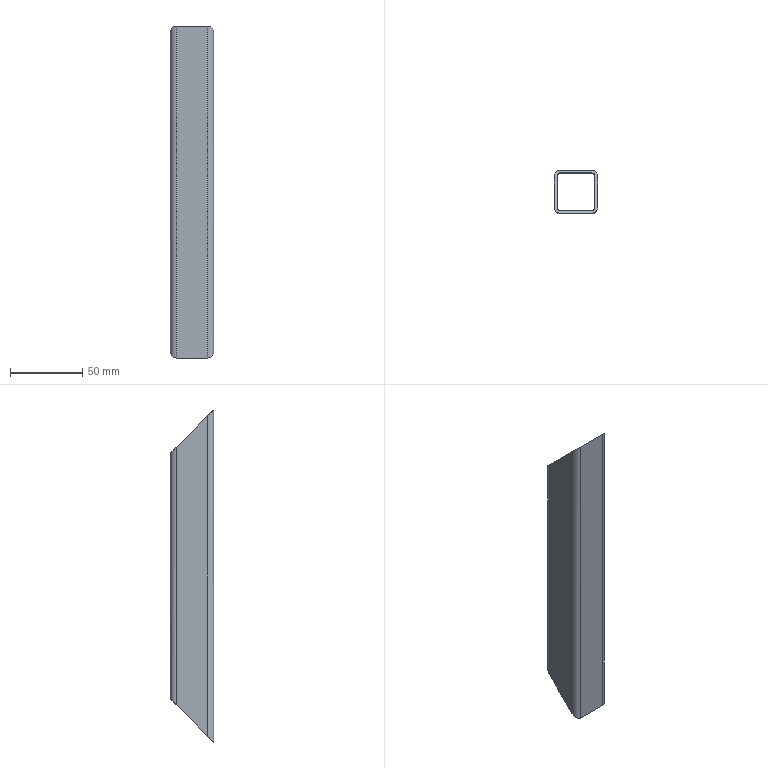Part | NX | features DATUM_CSYS 3, EXTRUDE 2, SKETCH 2, CPROJ 1 | 1 solid | 18 faces | box 30 x 30 x 230 mm | volume 42740 mm3 | plane 10 | cylinder 8 | commonest cylinder face diameters 4 x4 8 x4
STEP:
#1=CARTESIAN_POINT('',(13.,11.,26.));
#2=VERTEX_POINT('',#1);
#3=CARTESIAN_POINT('',(13.,11.,204.));
#4=VERTEX_POINT('',#3);
#5=CARTESIAN_POINT('',(13.,11.,0.));
#6=DIRECTION('',(0.,0.,-1.));
#7=VECTOR('',#6,1000.);
#8=LINE('',#5,#7);
#9=EDGE_CURVE('',#2,#4,#8,.F.);
#10=ORIENTED_EDGE('',*,*,#9,.T.);
#11=CARTESIAN_POINT('',(11.,13.,202.));
#12=VERTEX_POINT('',#11);
#13=CARTESIAN_POINT('',(11.,11.,204.));
#14=DIRECTION('',(0.,-0.7071,-0.7071));
#15=DIRECTION('',(0.,-0.7071,0.7071));
#16=AXIS2_PLACEMENT_3D('',#13,#14,#15);
#17=ELLIPSE('',#16,2.828,2.);
#18=EDGE_CURVE('',#4,#12,#17,.F.);
#19=ORIENTED_EDGE('',*,*,#18,.T.);
#20=CARTESIAN_POINT('',(11.,13.,28.));
#21=VERTEX_POINT('',#20);
#22=CARTESIAN_POINT('',(11.,13.,0.));
#23=DIRECTION('',(0.,0.,1.));
#24=VECTOR('',#23,1000.);
#25=LINE('',#22,#24);
#26=EDGE_CURVE('',#21,#12,#25,.T.);
#27=ORIENTED_EDGE('',*,*,#26,.F.);
#28=CARTESIAN_POINT('',(11.,11.,26.));
#29=DIRECTION('',(0.,-0.7071,0.7071));
#30=DIRECTION('',(0.,0.7071,0.7071));
#31=AXIS2_PLACEMENT_3D('',#28,#29,#30);
#32=ELLIPSE('',#31,2.828,2.);
#33=EDGE_CURVE('',#21,#2,#32,.F.);
#34=ORIENTED_EDGE('',*,*,#33,.T.);
#35=EDGE_LOOP('',(#10,#19,#27,#34));
#36=FACE_BOUND('',#35,.T.);
#37=CARTESIAN_POINT('',(11.,11.,0.));
#38=DIRECTION('',(0.,0.,1.));
#39=DIRECTION('',(1.,0.,0.));
#40=AXIS2_PLACEMENT_3D('',#37,#38,#39);
#41=CYLINDRICAL_SURFACE('',#40,2.);
#42=ADVANCED_FACE('',(#36),#41,.F.);
#43=CARTESIAN_POINT('',(13.,-11.,4.));
#44=VERTEX_POINT('',#43);
#45=CARTESIAN_POINT('',(13.,-11.,226.));
#46=VERTEX_POINT('',#45);
#47=CARTESIAN_POINT('',(13.,-11.,0.));
#48=DIRECTION('',(0.,0.,1.));
#49=VECTOR('',#48,1000.);
#50=LINE('',#47,#49);
#51=EDGE_CURVE('',#44,#46,#50,.T.);
#52=ORIENTED_EDGE('',*,*,#51,.T.);
#53=CARTESIAN_POINT('',(13.,102.,113.));
#54=DIRECTION('',(0.,0.7071,-0.7071));
#55=VECTOR('',#54,1000.);
#56=LINE('',#53,#55);
#57=EDGE_CURVE('',#46,#4,#56,.T.);
#58=ORIENTED_EDGE('',*,*,#57,.T.);
#59=ORIENTED_EDGE('',*,*,#9,.F.);
#60=CARTESIAN_POINT('',(13.,-13.,2.));
#61=DIRECTION('',(0.,-0.7071,-0.7071));
#62=VECTOR('',#61,1000.);
#63=LINE('',#60,#62);
#64=EDGE_CURVE('',#2,#44,#63,.T.);
#65=ORIENTED_EDGE('',*,*,#64,.T.);
#66=EDGE_LOOP('',(#52,#58,#59,#65));
#67=FACE_BOUND('',#66,.T.);
#68=CARTESIAN_POINT('',(13.,-11.,0.));
#69=DIRECTION('',(1.,0.,0.));
#70=DIRECTION('',(0.,0.,-1.));
#71=AXIS2_PLACEMENT_3D('',#68,#69,#70);
#72=PLANE('',#71);
#73=ADVANCED_FACE('',(#67),#72,.F.);
#74=CARTESIAN_POINT('',(11.,-13.,2.));
#75=VERTEX_POINT('',#74);
#76=CARTESIAN_POINT('',(11.,-13.,228.));
#77=VERTEX_POINT('',#76);
#78=CARTESIAN_POINT('',(11.,-13.,0.));
#79=DIRECTION('',(0.,0.,1.));
#80=VECTOR('',#79,1000.);
#81=LINE('',#78,#80);
#82=EDGE_CURVE('',#75,#77,#81,.T.);
#83=ORIENTED_EDGE('',*,*,#82,.T.);
#84=CARTESIAN_POINT('',(11.,-11.,226.));
#85=DIRECTION('',(0.,-0.7071,-0.7071));
#86=DIRECTION('',(0.,-0.7071,0.7071));
#87=AXIS2_PLACEMENT_3D('',#84,#85,#86);
#88=ELLIPSE('',#87,2.828,2.);
#89=EDGE_CURVE('',#77,#46,#88,.F.);
#90=ORIENTED_EDGE('',*,*,#89,.T.);
#91=ORIENTED_EDGE('',*,*,#51,.F.);
#92=CARTESIAN_POINT('',(11.,-11.,4.));
#93=DIRECTION('',(0.,-0.7071,0.7071));
#94=DIRECTION('',(0.,0.7071,0.7071));
#95=AXIS2_PLACEMENT_3D('',#92,#93,#94);
#96=ELLIPSE('',#95,2.828,2.);
#97=EDGE_CURVE('',#44,#75,#96,.F.);
#98=ORIENTED_EDGE('',*,*,#97,.T.);
#99=EDGE_LOOP('',(#83,#90,#91,#98));
#100=FACE_BOUND('',#99,.T.);
#101=CARTESIAN_POINT('',(11.,-11.,0.));
#102=DIRECTION('',(0.,0.,1.));
#103=DIRECTION('',(1.,0.,0.));
#104=AXIS2_PLACEMENT_3D('',#101,#102,#103);
#105=CYLINDRICAL_SURFACE('',#104,2.);
#106=ADVANCED_FACE('',(#100),#105,.F.);
#107=CARTESIAN_POINT('',(-11.,-13.,2.));
#108=VERTEX_POINT('',#107);
#109=CARTESIAN_POINT('',(-11.,-13.,228.));
#110=VERTEX_POINT('',#109);
#111=CARTESIAN_POINT('',(-11.,-13.,0.));
#112=DIRECTION('',(0.,0.,1.));
#113=VECTOR('',#112,1000.);
#114=LINE('',#111,#113);
#115=EDGE_CURVE('',#108,#110,#114,.T.);
#116=ORIENTED_EDGE('',*,*,#115,.T.);
#117=CARTESIAN_POINT('',(-11.,-13.,228.));
#118=DIRECTION('',(1.,0.,0.));
#119=VECTOR('',#118,1000.);
#120=LINE('',#117,#119);
#121=EDGE_CURVE('',#110,#77,#120,.T.);
#122=ORIENTED_EDGE('',*,*,#121,.T.);
#123=ORIENTED_EDGE('',*,*,#82,.F.);
#124=CARTESIAN_POINT('',(-11.,-13.,2.));
#125=DIRECTION('',(-1.,0.,0.));
#126=VECTOR('',#125,1000.);
#127=LINE('',#124,#126);
#128=EDGE_CURVE('',#75,#108,#127,.T.);
#129=ORIENTED_EDGE('',*,*,#128,.T.);
#130=EDGE_LOOP('',(#116,#122,#123,#129));
#131=FACE_BOUND('',#130,.T.);
#132=CARTESIAN_POINT('',(-11.,-13.,0.));
#133=DIRECTION('',(0.,-1.,0.));
#134=DIRECTION('',(1.,0.,0.));
#135=AXIS2_PLACEMENT_3D('',#132,#133,#134);
#136=PLANE('',#135);
#137=ADVANCED_FACE('',(#131),#136,.F.);
#138=CARTESIAN_POINT('',(-13.,-11.,4.));
#139=VERTEX_POINT('',#138);
#140=CARTESIAN_POINT('',(-13.,-11.,226.));
#141=VERTEX_POINT('',#140);
#142=CARTESIAN_POINT('',(-13.,-11.,0.));
#143=DIRECTION('',(0.,0.,1.));
#144=VECTOR('',#143,1000.);
#145=LINE('',#142,#144);
#146=EDGE_CURVE('',#139,#141,#145,.T.);
#147=ORIENTED_EDGE('',*,*,#146,.T.);
#148=CARTESIAN_POINT('',(-11.,-11.,226.));
#149=DIRECTION('',(0.,-0.7071,-0.7071));
#150=DIRECTION('',(0.,-0.7071,0.7071));
#151=AXIS2_PLACEMENT_3D('',#148,#149,#150);
#152=ELLIPSE('',#151,2.828,2.);
#153=EDGE_CURVE('',#141,#110,#152,.F.);
#154=ORIENTED_EDGE('',*,*,#153,.T.);
#155=ORIENTED_EDGE('',*,*,#115,.F.);
#156=CARTESIAN_POINT('',(-11.,-11.,4.));
#157=DIRECTION('',(0.,-0.7071,0.7071));
#158=DIRECTION('',(0.,0.7071,0.7071));
#159=AXIS2_PLACEMENT_3D('',#156,#157,#158);
#160=ELLIPSE('',#159,2.828,2.);
#161=EDGE_CURVE('',#108,#139,#160,.F.);
#162=ORIENTED_EDGE('',*,*,#161,.T.);
#163=EDGE_LOOP('',(#147,#154,#155,#162));
#164=FACE_BOUND('',#163,.T.);
#165=CARTESIAN_POINT('',(-11.,-11.,0.));
#166=DIRECTION('',(0.,0.,1.));
#167=DIRECTION('',(1.,0.,0.));
#168=AXIS2_PLACEMENT_3D('',#165,#166,#167);
#169=CYLINDRICAL_SURFACE('',#168,2.);
#170=ADVANCED_FACE('',(#164),#169,.F.);
#171=CARTESIAN_POINT('',(-13.,11.,26.));
#172=VERTEX_POINT('',#171);
#173=CARTESIAN_POINT('',(-13.,11.,204.));
#174=VERTEX_POINT('',#173);
#175=CARTESIAN_POINT('',(-13.,11.,0.));
#176=DIRECTION('',(0.,0.,1.));
#177=VECTOR('',#176,1000.);
#178=LINE('',#175,#177);
#179=EDGE_CURVE('',#172,#174,#178,.T.);
#180=ORIENTED_EDGE('',*,*,#179,.T.);
#181=CARTESIAN_POINT('',(-13.,113.,102.));
#182=DIRECTION('',(0.,-0.7071,0.7071));
#183=VECTOR('',#182,1000.);
#184=LINE('',#181,#183);
#185=EDGE_CURVE('',#174,#141,#184,.T.);
#186=ORIENTED_EDGE('',*,*,#185,.T.);
#187=ORIENTED_EDGE('',*,*,#146,.F.);
#188=CARTESIAN_POINT('',(-13.,-2.,13.));
#189=DIRECTION('',(0.,0.7071,0.7071));
#190=VECTOR('',#189,1000.);
#191=LINE('',#188,#190);
#192=EDGE_CURVE('',#139,#172,#191,.T.);
#193=ORIENTED_EDGE('',*,*,#192,.T.);
#194=EDGE_LOOP('',(#180,#186,#187,#193));
#195=FACE_BOUND('',#194,.T.);
#196=CARTESIAN_POINT('',(-13.,11.,0.));
#197=DIRECTION('',(-1.,0.,0.));
#198=DIRECTION('',(0.,-1.,0.));
#199=AXIS2_PLACEMENT_3D('',#196,#197,#198);
#200=PLANE('',#199);
#201=ADVANCED_FACE('',(#195),#200,.F.);
#202=CARTESIAN_POINT('',(-11.,13.,28.));
#203=VERTEX_POINT('',#202);
#204=CARTESIAN_POINT('',(-11.,13.,202.));
#205=VERTEX_POINT('',#204);
#206=CARTESIAN_POINT('',(-11.,13.,0.));
#207=DIRECTION('',(0.,0.,1.));
#208=VECTOR('',#207,1000.);
#209=LINE('',#206,#208);
#210=EDGE_CURVE('',#203,#205,#209,.T.);
#211=ORIENTED_EDGE('',*,*,#210,.T.);
#212=CARTESIAN_POINT('',(-11.,11.,204.));
#213=DIRECTION('',(0.,-0.7071,-0.7071));
#214=DIRECTION('',(0.,-0.7071,0.7071));
#215=AXIS2_PLACEMENT_3D('',#212,#213,#214);
#216=ELLIPSE('',#215,2.828,2.);
#217=EDGE_CURVE('',#205,#174,#216,.F.);
#218=ORIENTED_EDGE('',*,*,#217,.T.);
#219=ORIENTED_EDGE('',*,*,#179,.F.);
#220=CARTESIAN_POINT('',(-11.,11.,26.));
#221=DIRECTION('',(0.,-0.7071,0.7071));
#222=DIRECTION('',(0.,0.7071,0.7071));
#223=AXIS2_PLACEMENT_3D('',#220,#221,#222);
#224=ELLIPSE('',#223,2.828,2.);
#225=EDGE_CURVE('',#172,#203,#224,.F.);
#226=ORIENTED_EDGE('',*,*,#225,.T.);
#227=EDGE_LOOP('',(#211,#218,#219,#226));
#228=FACE_BOUND('',#227,.T.);
#229=CARTESIAN_POINT('',(-11.,11.,0.));
#230=DIRECTION('',(0.,0.,1.));
#231=DIRECTION('',(1.,0.,0.));
#232=AXIS2_PLACEMENT_3D('',#229,#230,#231);
#233=CYLINDRICAL_SURFACE('',#232,2.);
#234=ADVANCED_FACE('',(#228),#233,.F.);
#235=ORIENTED_EDGE('',*,*,#26,.T.);
#236=CARTESIAN_POINT('',(11.,13.,202.));
#237=DIRECTION('',(-1.,0.,0.));
#238=VECTOR('',#237,1000.);
#239=LINE('',#236,#238);
#240=EDGE_CURVE('',#12,#205,#239,.T.);
#241=ORIENTED_EDGE('',*,*,#240,.T.);
#242=ORIENTED_EDGE('',*,*,#210,.F.);
#243=CARTESIAN_POINT('',(11.,13.,28.));
#244=DIRECTION('',(1.,0.,0.));
#245=VECTOR('',#244,1000.);
#246=LINE('',#243,#245);
#247=EDGE_CURVE('',#203,#21,#246,.T.);
#248=ORIENTED_EDGE('',*,*,#247,.T.);
#249=EDGE_LOOP('',(#235,#241,#242,#248));
#250=FACE_BOUND('',#249,.T.);
#251=CARTESIAN_POINT('',(11.,13.,0.));
#252=DIRECTION('',(0.,1.,0.));
#253=DIRECTION('',(-1.,0.,0.));
#254=AXIS2_PLACEMENT_3D('',#251,#252,#253);
#255=PLANE('',#254);
#256=ADVANCED_FACE('',(#250),#255,.F.);
#257=CARTESIAN_POINT('',(-15.,11.,26.));
#258=VERTEX_POINT('',#257);
#259=CARTESIAN_POINT('',(-11.,15.,30.));
#260=VERTEX_POINT('',#259);
#261=CARTESIAN_POINT('',(-11.,11.,26.));
#262=DIRECTION('',(0.,-0.7071,0.7071));
#263=DIRECTION('',(0.,0.7071,0.7071));
#264=AXIS2_PLACEMENT_3D('',#261,#262,#263);
#265=ELLIPSE('',#264,5.657,4.);
#266=EDGE_CURVE('',#258,#260,#265,.F.);
#267=ORIENTED_EDGE('',*,*,#266,.T.);
#268=CARTESIAN_POINT('',(11.,15.,30.));
#269=VERTEX_POINT('',#268);
#270=CARTESIAN_POINT('',(-29.5,15.,30.));
#271=DIRECTION('',(1.,0.,0.));
#272=VECTOR('',#271,1000.);
#273=LINE('',#270,#272);
#274=EDGE_CURVE('',#260,#269,#273,.T.);
#275=ORIENTED_EDGE('',*,*,#274,.T.);
#276=CARTESIAN_POINT('',(15.,11.,26.));
#277=VERTEX_POINT('',#276);
#278=CARTESIAN_POINT('',(11.,11.,26.));
#279=DIRECTION('',(0.,-0.7071,0.7071));
#280=DIRECTION('',(0.,0.7071,0.7071));
#281=AXIS2_PLACEMENT_3D('',#278,#279,#280);
#282=ELLIPSE('',#281,5.657,4.);
#283=EDGE_CURVE('',#269,#277,#282,.F.);
#284=ORIENTED_EDGE('',*,*,#283,.T.);
#285=CARTESIAN_POINT('',(15.,-11.,4.));
#286=VERTEX_POINT('',#285);
#287=CARTESIAN_POINT('',(15.,15.,30.));
#288=DIRECTION('',(0.,-0.7071,-0.7071));
#289=VECTOR('',#288,1000.);
#290=LINE('',#287,#289);
#291=EDGE_CURVE('',#277,#286,#290,.T.);
#292=ORIENTED_EDGE('',*,*,#291,.T.);
#293=CARTESIAN_POINT('',(11.,-15.,0.));
#294=VERTEX_POINT('',#293);
#295=CARTESIAN_POINT('',(11.,-11.,4.));
#296=DIRECTION('',(0.,-0.7071,0.7071));
#297=DIRECTION('',(0.,0.7071,0.7071));
#298=AXIS2_PLACEMENT_3D('',#295,#296,#297);
#299=ELLIPSE('',#298,5.657,4.);
#300=EDGE_CURVE('',#286,#294,#299,.F.);
#301=ORIENTED_EDGE('',*,*,#300,.T.);
#302=CARTESIAN_POINT('',(-11.,-15.,0.));
#303=VERTEX_POINT('',#302);
#304=CARTESIAN_POINT('',(-11.,-15.,0.));
#305=DIRECTION('',(1.,0.,0.));
#306=VECTOR('',#305,1000.);
#307=LINE('',#304,#306);
#308=EDGE_CURVE('',#303,#294,#307,.T.);
#309=ORIENTED_EDGE('',*,*,#308,.F.);
#310=CARTESIAN_POINT('',(-15.,-11.,4.));
#311=VERTEX_POINT('',#310);
#312=CARTESIAN_POINT('',(-11.,-11.,4.));
#313=DIRECTION('',(0.,-0.7071,0.7071));
#314=DIRECTION('',(0.,0.7071,0.7071));
#315=AXIS2_PLACEMENT_3D('',#312,#313,#314);
#316=ELLIPSE('',#315,5.657,4.);
#317=EDGE_CURVE('',#303,#311,#316,.F.);
#318=ORIENTED_EDGE('',*,*,#317,.T.);
#319=CARTESIAN_POINT('',(-15.,-2.,13.));
#320=DIRECTION('',(0.,0.7071,0.7071));
#321=VECTOR('',#320,1000.);
#322=LINE('',#319,#321);
#323=EDGE_CURVE('',#311,#258,#322,.T.);
#324=ORIENTED_EDGE('',*,*,#323,.T.);
#325=EDGE_LOOP('',(#267,#275,#284,#292,#301,#309,#318,#324));
#326=FACE_BOUND('',#325,.T.);
#327=ORIENTED_EDGE('',*,*,#225,.F.);
#328=ORIENTED_EDGE('',*,*,#192,.F.);
#329=ORIENTED_EDGE('',*,*,#161,.F.);
#330=ORIENTED_EDGE('',*,*,#128,.F.);
#331=ORIENTED_EDGE('',*,*,#97,.F.);
#332=ORIENTED_EDGE('',*,*,#64,.F.);
#333=ORIENTED_EDGE('',*,*,#33,.F.);
#334=ORIENTED_EDGE('',*,*,#247,.F.);
#335=EDGE_LOOP('',(#327,#328,#329,#330,#331,#332,#333,#334));
#336=FACE_BOUND('',#335,.T.);
#337=CARTESIAN_POINT('',(-29.5,15.,30.));
#338=DIRECTION('',(0.,-0.7071,0.7071));
#339=DIRECTION('',(0.,-0.7071,-0.7071));
#340=AXIS2_PLACEMENT_3D('',#337,#338,#339);
#341=PLANE('',#340);
#342=ADVANCED_FACE('',(#326,#336),#341,.F.);
#343=CARTESIAN_POINT('',(-11.,15.,200.));
#344=VERTEX_POINT('',#343);
#345=CARTESIAN_POINT('',(-15.,11.,204.));
#346=VERTEX_POINT('',#345);
#347=CARTESIAN_POINT('',(-11.,11.,204.));
#348=DIRECTION('',(0.,-0.7071,-0.7071));
#349=DIRECTION('',(0.,-0.7071,0.7071));
#350=AXIS2_PLACEMENT_3D('',#347,#348,#349);
#351=ELLIPSE('',#350,5.657,4.);
#352=EDGE_CURVE('',#344,#346,#351,.F.);
#353=ORIENTED_EDGE('',*,*,#352,.T.);
#354=CARTESIAN_POINT('',(-15.,-11.,226.));
#355=VERTEX_POINT('',#354);
#356=CARTESIAN_POINT('',(-15.,113.,102.));
#357=DIRECTION('',(0.,-0.7071,0.7071));
#358=VECTOR('',#357,1000.);
#359=LINE('',#356,#358);
#360=EDGE_CURVE('',#346,#355,#359,.T.);
#361=ORIENTED_EDGE('',*,*,#360,.T.);
#362=CARTESIAN_POINT('',(-11.,-15.,230.));
#363=VERTEX_POINT('',#362);
#364=CARTESIAN_POINT('',(-11.,-11.,226.));
#365=DIRECTION('',(0.,-0.7071,-0.7071));
#366=DIRECTION('',(0.,-0.7071,0.7071));
#367=AXIS2_PLACEMENT_3D('',#364,#365,#366);
#368=ELLIPSE('',#367,5.657,4.);
#369=EDGE_CURVE('',#355,#363,#368,.F.);
#370=ORIENTED_EDGE('',*,*,#369,.T.);
#371=CARTESIAN_POINT('',(11.,-15.,230.));
#372=VERTEX_POINT('',#371);
#373=CARTESIAN_POINT('',(-11.,-15.,230.));
#374=DIRECTION('',(1.,0.,0.));
#375=VECTOR('',#374,1000.);
#376=LINE('',#373,#375);
#377=EDGE_CURVE('',#363,#372,#376,.T.);
#378=ORIENTED_EDGE('',*,*,#377,.T.);
#379=CARTESIAN_POINT('',(15.,-11.,226.));
#380=VERTEX_POINT('',#379);
#381=CARTESIAN_POINT('',(11.,-11.,226.));
#382=DIRECTION('',(0.,-0.7071,-0.7071));
#383=DIRECTION('',(0.,-0.7071,0.7071));
#384=AXIS2_PLACEMENT_3D('',#381,#382,#383);
#385=ELLIPSE('',#384,5.657,4.);
#386=EDGE_CURVE('',#372,#380,#385,.F.);
#387=ORIENTED_EDGE('',*,*,#386,.T.);
#388=CARTESIAN_POINT('',(15.,11.,204.));
#389=VERTEX_POINT('',#388);
#390=CARTESIAN_POINT('',(15.,-15.,230.));
#391=DIRECTION('',(0.,0.7071,-0.7071));
#392=VECTOR('',#391,1000.);
#393=LINE('',#390,#392);
#394=EDGE_CURVE('',#380,#389,#393,.T.);
#395=ORIENTED_EDGE('',*,*,#394,.T.);
#396=CARTESIAN_POINT('',(11.,15.,200.));
#397=VERTEX_POINT('',#396);
#398=CARTESIAN_POINT('',(11.,11.,204.));
#399=DIRECTION('',(0.,-0.7071,-0.7071));
#400=DIRECTION('',(0.,-0.7071,0.7071));
#401=AXIS2_PLACEMENT_3D('',#398,#399,#400);
#402=ELLIPSE('',#401,5.657,4.);
#403=EDGE_CURVE('',#389,#397,#402,.F.);
#404=ORIENTED_EDGE('',*,*,#403,.T.);
#405=CARTESIAN_POINT('',(-29.5,15.,200.));
#406=DIRECTION('',(1.,0.,0.));
#407=VECTOR('',#406,1000.);
#408=LINE('',#405,#407);
#409=EDGE_CURVE('',#344,#397,#408,.T.);
#410=ORIENTED_EDGE('',*,*,#409,.F.);
#411=EDGE_LOOP('',(#353,#361,#370,#378,#387,#395,#404,#410));
#412=FACE_BOUND('',#411,.T.);
#413=ORIENTED_EDGE('',*,*,#18,.F.);
#414=ORIENTED_EDGE('',*,*,#57,.F.);
#415=ORIENTED_EDGE('',*,*,#89,.F.);
#416=ORIENTED_EDGE('',*,*,#121,.F.);
#417=ORIENTED_EDGE('',*,*,#153,.F.);
#418=ORIENTED_EDGE('',*,*,#185,.F.);
#419=ORIENTED_EDGE('',*,*,#217,.F.);
#420=ORIENTED_EDGE('',*,*,#240,.F.);
#421=EDGE_LOOP('',(#413,#414,#415,#416,#417,#418,#419,#420));
#422=FACE_BOUND('',#421,.T.);
#423=CARTESIAN_POINT('',(-29.5,-15.,230.));
#424=DIRECTION('',(0.,-0.7071,-0.7071));
#425=DIRECTION('',(0.,0.7071,-0.7071));
#426=AXIS2_PLACEMENT_3D('',#423,#424,#425);
#427=PLANE('',#426);
#428=ADVANCED_FACE('',(#412,#422),#427,.F.);
#429=CARTESIAN_POINT('',(-11.,15.,0.));
#430=DIRECTION('',(0.,0.,1.));
#431=VECTOR('',#430,1000.);
#432=LINE('',#429,#431);
#433=EDGE_CURVE('',#260,#344,#432,.T.);
#434=ORIENTED_EDGE('',*,*,#433,.T.);
#435=ORIENTED_EDGE('',*,*,#409,.T.);
#436=CARTESIAN_POINT('',(11.,15.,0.));
#437=DIRECTION('',(0.,0.,1.));
#438=VECTOR('',#437,1000.);
#439=LINE('',#436,#438);
#440=EDGE_CURVE('',#269,#397,#439,.T.);
#441=ORIENTED_EDGE('',*,*,#440,.F.);
#442=ORIENTED_EDGE('',*,*,#274,.F.);
#443=EDGE_LOOP('',(#434,#435,#441,#442));
#444=FACE_BOUND('',#443,.T.);
#445=CARTESIAN_POINT('',(11.,15.,0.));
#446=DIRECTION('',(0.,1.,0.));
#447=DIRECTION('',(-1.,0.,0.));
#448=AXIS2_PLACEMENT_3D('',#445,#446,#447);
#449=PLANE('',#448);
#450=ADVANCED_FACE('',(#444),#449,.T.);
#451=ORIENTED_EDGE('',*,*,#352,.F.);
#452=ORIENTED_EDGE('',*,*,#433,.F.);
#453=ORIENTED_EDGE('',*,*,#266,.F.);
#454=CARTESIAN_POINT('',(-15.,11.,0.));
#455=DIRECTION('',(0.,0.,1.));
#456=VECTOR('',#455,1000.);
#457=LINE('',#454,#456);
#458=EDGE_CURVE('',#258,#346,#457,.T.);
#459=ORIENTED_EDGE('',*,*,#458,.T.);
#460=EDGE_LOOP('',(#451,#452,#453,#459));
#461=FACE_BOUND('',#460,.T.);
#462=CARTESIAN_POINT('',(-11.,11.,0.));
#463=DIRECTION('',(0.,0.,1.));
#464=DIRECTION('',(1.,0.,0.));
#465=AXIS2_PLACEMENT_3D('',#462,#463,#464);
#466=CYLINDRICAL_SURFACE('',#465,4.);
#467=ADVANCED_FACE('',(#461),#466,.T.);
#468=ORIENTED_EDGE('',*,*,#360,.F.);
#469=ORIENTED_EDGE('',*,*,#458,.F.);
#470=ORIENTED_EDGE('',*,*,#323,.F.);
#471=CARTESIAN_POINT('',(-15.,-11.,0.));
#472=DIRECTION('',(0.,0.,1.));
#473=VECTOR('',#472,1000.);
#474=LINE('',#471,#473);
#475=EDGE_CURVE('',#311,#355,#474,.T.);
#476=ORIENTED_EDGE('',*,*,#475,.T.);
#477=EDGE_LOOP('',(#468,#469,#470,#476));
#478=FACE_BOUND('',#477,.T.);
#479=CARTESIAN_POINT('',(-15.,11.,0.));
#480=DIRECTION('',(-1.,0.,0.));
#481=DIRECTION('',(0.,-1.,0.));
#482=AXIS2_PLACEMENT_3D('',#479,#480,#481);
#483=PLANE('',#482);
#484=ADVANCED_FACE('',(#478),#483,.T.);
#485=ORIENTED_EDGE('',*,*,#369,.F.);
#486=ORIENTED_EDGE('',*,*,#475,.F.);
#487=ORIENTED_EDGE('',*,*,#317,.F.);
#488=CARTESIAN_POINT('',(-11.,-15.,0.));
#489=DIRECTION('',(0.,0.,1.));
#490=VECTOR('',#489,1000.);
#491=LINE('',#488,#490);
#492=EDGE_CURVE('',#303,#363,#491,.T.);
#493=ORIENTED_EDGE('',*,*,#492,.T.);
#494=EDGE_LOOP('',(#485,#486,#487,#493));
#495=FACE_BOUND('',#494,.T.);
#496=CARTESIAN_POINT('',(-11.,-11.,0.));
#497=DIRECTION('',(0.,0.,1.));
#498=DIRECTION('',(1.,0.,0.));
#499=AXIS2_PLACEMENT_3D('',#496,#497,#498);
#500=CYLINDRICAL_SURFACE('',#499,4.);
#501=ADVANCED_FACE('',(#495),#500,.T.);
#502=ORIENTED_EDGE('',*,*,#377,.F.);
#503=ORIENTED_EDGE('',*,*,#492,.F.);
#504=ORIENTED_EDGE('',*,*,#308,.T.);
#505=CARTESIAN_POINT('',(11.,-15.,0.));
#506=DIRECTION('',(0.,0.,1.));
#507=VECTOR('',#506,1000.);
#508=LINE('',#505,#507);
#509=EDGE_CURVE('',#294,#372,#508,.T.);
#510=ORIENTED_EDGE('',*,*,#509,.T.);
#511=EDGE_LOOP('',(#502,#503,#504,#510));
#512=FACE_BOUND('',#511,.T.);
#513=CARTESIAN_POINT('',(-11.,-15.,0.));
#514=DIRECTION('',(0.,-1.,0.));
#515=DIRECTION('',(1.,0.,0.));
#516=AXIS2_PLACEMENT_3D('',#513,#514,#515);
#517=PLANE('',#516);
#518=ADVANCED_FACE('',(#512),#517,.T.);
#519=ORIENTED_EDGE('',*,*,#386,.F.);
#520=ORIENTED_EDGE('',*,*,#509,.F.);
#521=ORIENTED_EDGE('',*,*,#300,.F.);
#522=CARTESIAN_POINT('',(15.,-11.,0.));
#523=DIRECTION('',(0.,0.,1.));
#524=VECTOR('',#523,1000.);
#525=LINE('',#522,#524);
#526=EDGE_CURVE('',#286,#380,#525,.T.);
#527=ORIENTED_EDGE('',*,*,#526,.T.);
#528=EDGE_LOOP('',(#519,#520,#521,#527));
#529=FACE_BOUND('',#528,.T.);
#530=CARTESIAN_POINT('',(11.,-11.,0.));
#531=DIRECTION('',(0.,0.,1.));
#532=DIRECTION('',(1.,0.,0.));
#533=AXIS2_PLACEMENT_3D('',#530,#531,#532);
#534=CYLINDRICAL_SURFACE('',#533,4.);
#535=ADVANCED_FACE('',(#529),#534,.T.);
#536=ORIENTED_EDGE('',*,*,#394,.F.);
#537=ORIENTED_EDGE('',*,*,#526,.F.);
#538=ORIENTED_EDGE('',*,*,#291,.F.);
#539=CARTESIAN_POINT('',(15.,11.,0.));
#540=DIRECTION('',(0.,0.,1.));
#541=VECTOR('',#540,1000.);
#542=LINE('',#539,#541);
#543=EDGE_CURVE('',#277,#389,#542,.T.);
#544=ORIENTED_EDGE('',*,*,#543,.T.);
#545=EDGE_LOOP('',(#536,#537,#538,#544));
#546=FACE_BOUND('',#545,.T.);
#547=CARTESIAN_POINT('',(15.,-11.,0.));
#548=DIRECTION('',(1.,0.,0.));
#549=DIRECTION('',(0.,0.,-1.));
#550=AXIS2_PLACEMENT_3D('',#547,#548,#549);
#551=PLANE('',#550);
#552=ADVANCED_FACE('',(#546),#551,.T.);
#553=ORIENTED_EDGE('',*,*,#403,.F.);
#554=ORIENTED_EDGE('',*,*,#543,.F.);
#555=ORIENTED_EDGE('',*,*,#283,.F.);
#556=ORIENTED_EDGE('',*,*,#440,.T.);
#557=EDGE_LOOP('',(#553,#554,#555,#556));
#558=FACE_BOUND('',#557,.T.);
#559=CARTESIAN_POINT('',(11.,11.,0.));
#560=DIRECTION('',(0.,0.,1.));
#561=DIRECTION('',(1.,0.,0.));
#562=AXIS2_PLACEMENT_3D('',#559,#560,#561);
#563=CYLINDRICAL_SURFACE('',#562,4.);
#564=ADVANCED_FACE('',(#558),#563,.T.);
#565=CLOSED_SHELL('',(#42,#73,#106,#137,#170,#201,#234,#256,#342,#428,#450,#467,#484,#501,#518,#535,#552,#564));
#566=MANIFOLD_SOLID_BREP('',#565);
#567=(LENGTH_UNIT()NAMED_UNIT(*)SI_UNIT(.MILLI.,.METRE.));
#568=UNCERTAINTY_MEASURE_WITH_UNIT(LENGTH_MEASURE(0.00001),#567,'','');
#569=(NAMED_UNIT(*)PLANE_ANGLE_UNIT()SI_UNIT($,.RADIAN.));
#570=(NAMED_UNIT(*)SI_UNIT($,.STERADIAN.)SOLID_ANGLE_UNIT());
#571=(GEOMETRIC_REPRESENTATION_CONTEXT(3)GLOBAL_UNCERTAINTY_ASSIGNED_CONTEXT((#568))GLOBAL_UNIT_ASSIGNED_CONTEXT((#567,#569,#570))REPRESENTATION_CONTEXT('',''));
#572=ADVANCED_BREP_SHAPE_REPRESENTATION('',(#566),#571);